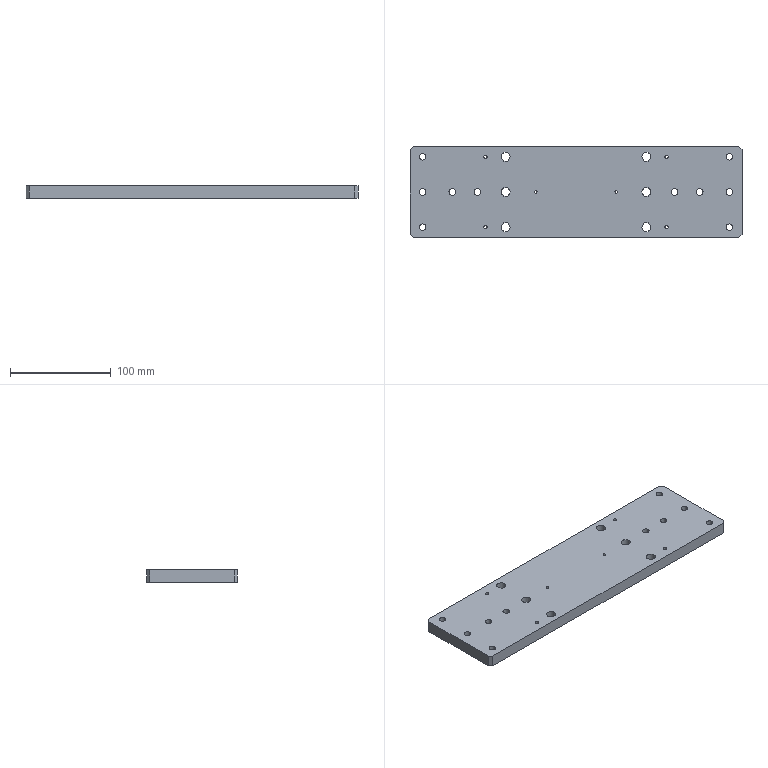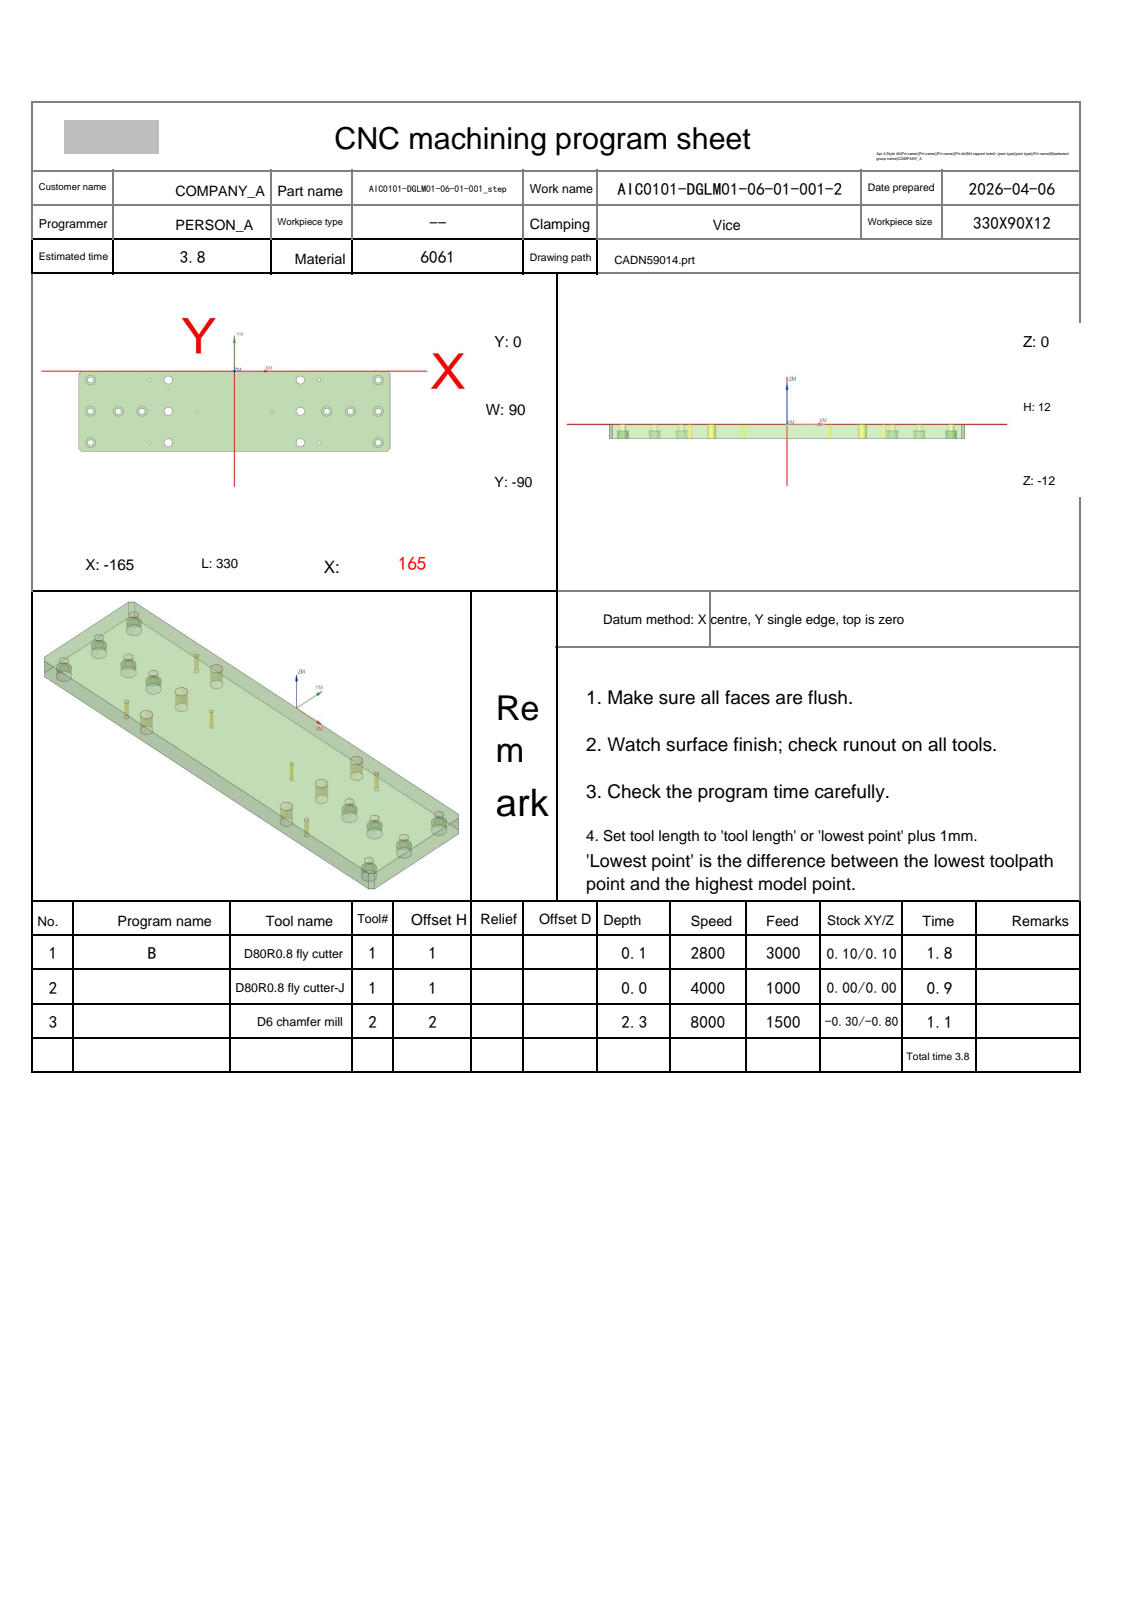NC program | NX | posted by the shop | part box 330 x 90 x 12 mm
Whole program:
%
O0001
(Machine time: 4.35 MIN)
(===Total Tool:2===)
(T1=D80R0.8 fly cutter D=80.  R=0.8  D-  H01 Z=0.    )
(T2=D6 chamfer mill   D=6.   R=0.   D-  H02 Z=-2.3  )
G80 G90 G17 G49 G40
G91 G28 Z0
M01
N1 T01 M06
(D80R0.8 fly cutter  D=80. R=0.8 H=01 ce=0.10 di=0.10)
G00 G90 G54 X-217.097 Y-23.903 M03 S2800
G43 H01 Z20.
M08
Z4.517
G01 Z2.517 F3000.
X-205.097
X197.897
G02 X205.097 Y-31.103 I0.0 J-7.2
G01 Y-50.737
G02 X197.097 Y-58.737 I-8. J0.0
G01 X-205.097
X-217.097
Z4.517
G00 Y-23.903
Z4.033
G01 Z2.033
X-205.097
X197.897
G02 X205.097 Y-31.103 I0.0 J-7.2
G01 Y-50.737
G02 X197.097 Y-58.737 I-8. J0.0
G01 X-205.097
X-217.097
Z4.033
G00 Y-23.903
Z3.55
G01 Z1.55
X-205.097
X197.897
G02 X205.097 Y-31.103 I0.0 J-7.2
G01 Y-50.737
G02 X197.097 Y-58.737 I-8. J0.0
G01 X-205.097
X-217.097
Z3.55
G00 Y-23.903
Z3.067
G01 Z1.067
X-205.097
X197.897
G02 X205.097 Y-31.103 I0.0 J-7.2
G01 Y-50.737
G02 X197.097 Y-58.737 I-8. J0.0
G01 X-205.097
X-217.097
Z3.067
G00 Y-23.903
Z2.583
G01 Z.583
X-205.097
X197.897
G02 X205.097 Y-31.103 I0.0 J-7.2
G01 Y-50.737
G02 X197.097 Y-58.737 I-8. J0.0
G01 X-205.097
X-217.097
Z2.583
G00 Y-23.903
Z2.1
G01 Z.1
X-205.097
X197.897
G02 X205.097 Y-31.103 I0.0 J-7.2
G01 Y-50.737
G02 X197.097 Y-58.737 I-8. J0.0
G01 X-205.097
X-217.097
Z2.1
G00 Z20.
G91 G28 Z0.0
M05
M09
G91 G28 Z0.0
M01
N2 T01 M06
(D80R0.8 fly cutter-J  D=80. R=0.8 H=01 ce=0.00 di=0.00)
G00 G90 G54 X-216.999 Y-24.001 M03 S4000
G43 H01 Z20.
M08
Z2.
G01 Z0.0 F1000.
X-204.999
X197.799
G02 X204.999 Y-31.201 I0.0 J-7.2
G01 Y-50.639
G02 X196.999 Y-58.639 I-8. J0.0
G01 X-204.999
X-216.999
Z2.
G00 Z20.
G91 G28 Z0.0
M05
M09
G91 G28 Z0.0
M01
N3 T02 M06
(D6 chamfer mill  D=6. R=0. H=02 ce=0.00 di=0.00)
G00 G90 G54 X-40. Y-45. M03 S8000
G43 H02 Z20.
M08
G98 G81 X-40. Y-45. Z-1.75 R3. F1000.
X40.
G80
G00 Z20.
G00 G90 X-90. Y-10. M03 S8000
Z20.
G98 G81 X-90. Y-10. Z-2.2 R3. F1000.
Y-80.
X90.
Y-10.
G80
G00 Z20.
G00 G90 X-151.993 Y-11.087 M03 S8000
Z20.
Z-.9
G01 Z-1.4 F1200.
X-151.8 Y-11.5
G03 X-150.3 Y-10. I0.0 J1.5
X-152.5 Y-7.8 I-2.2 J0.0
X-154.7 Y-10. I0.0 J-2.2
X-152.5 Y-12.2 I2.2 J0.0
X-150.3 Y-10. I0.0 J2.2
X-151.8 Y-8.5 I-1.5 J0.0
G01 X-151.993 Y-8.913
Z-.9
G00 Z20.
Y-46.087
Z-.9
G01 Z-1.4
X-151.8 Y-46.5
G03 X-150.3 Y-45. I0.0 J1.5
X-152.5 Y-42.8 I-2.2 J0.0
X-154.7 Y-45. I0.0 J-2.2
X-152.5 Y-47.2 I2.2 J0.0
X-150.3 Y-45. I0.0 J2.2
X-151.8 Y-43.5 I-1.5 J0.0
G01 X-151.993 Y-43.913
Z-.9
G00 Z20.
Y-81.087
Z-.9
G01 Z-1.4
X-151.8 Y-81.5
G03 X-150.3 Y-80. I0.0 J1.5
X-152.5 Y-77.8 I-2.2 J0.0
X-154.7 Y-80. I0.0 J-2.2
X-152.5 Y-82.2 I2.2 J0.0
X-150.3 Y-80. I0.0 J2.2
X-151.8 Y-78.5 I-1.5 J0.0
G01 X-151.993 Y-78.913
Z-.9
G00 Z20.
X-122.493 Y-46.087
Z-.9
G01 Z-1.4
X-122.3 Y-46.5
G03 X-120.8 Y-45. I0.0 J1.5
X-123. Y-42.8 I-2.2 J0.0
X-125.2 Y-45. I0.0 J-2.2
X-123. Y-47.2 I2.2 J0.0
X-120.8 Y-45. I0.0 J2.2
X-122.3 Y-43.5 I-1.5 J0.0
G01 X-122.493 Y-43.913
Z-.9
G00 Z20.
X-97.493 Y-46.087
Z-.9
G01 Z-1.4
X-97.3 Y-46.5
G03 X-95.8 Y-45. I0.0 J1.5
X-98. Y-42.8 I-2.2 J0.0
X-100.2 Y-45. I0.0 J-2.2
X-98. Y-47.2 I2.2 J0.0
X-95.8 Y-45. I0.0 J2.2
X-97.3 Y-43.5 I-1.5 J0.0
G01 X-97.493 Y-43.913
Z-.9
G00 Z20.
X98.507 Y-46.087
Z-.9
G01 Z-1.4
X98.7 Y-46.5
G03 X100.2 Y-45. I0.0 J1.5
X98. Y-42.8 I-2.2 J0.0
X95.8 Y-45. I0.0 J-2.2
X98. Y-47.2 I2.2 J0.0
X100.2 Y-45. I0.0 J2.2
X98.7 Y-43.5 I-1.5 J0.0
G01 X98.507 Y-43.913
Z-.9
G00 Z20.
X123.507 Y-46.087
Z-.9
G01 Z-1.4
X123.7 Y-46.5
G03 X125.2 Y-45. I0.0 J1.5
X123. Y-42.8 I-2.2 J0.0
X120.8 Y-45. I0.0 J-2.2
X123. Y-47.2 I2.2 J0.0
X125.2 Y-45. I0.0 J2.2
X123.7 Y-43.5 I-1.5 J0.0
G01 X123.507 Y-43.913
Z-.9
G00 Z20.
X153.007 Y-81.087
Z-.9
G01 Z-1.4
X153.2 Y-81.5
G03 X154.7 Y-80. I0.0 J1.5
X152.5 Y-77.8 I-2.2 J0.0
X150.3 Y-80. I0.0 J-2.2
X152.5 Y-82.2 I2.2 J0.0
X154.7 Y-80. I0.0 J2.2
X153.2 Y-78.5 I-1.5 J0.0
G01 X153.007 Y-78.913
Z-.9
G00 Z20.
Y-46.087
Z-.9
G01 Z-1.4
X153.2 Y-46.5
G03 X154.7 Y-45. I0.0 J1.5
X152.5 Y-42.8 I-2.2 J0.0
X150.3 Y-45. I0.0 J-2.2
X152.5 Y-47.2 I2.2 J0.0
X154.7 Y-45. I0.0 J2.2
X153.2 Y-43.5 I-1.5 J0.0
G01 X153.007 Y-43.913
Z-.9
G00 Z20.
Y-11.087
Z-.9
G01 Z-1.4
X153.2 Y-11.5
G03 X154.7 Y-10. I0.0 J1.5
X152.5 Y-7.8 I-2.2 J0.0
X150.3 Y-10. I0.0 J-2.2
X152.5 Y-12.2 I2.2 J0.0
X154.7 Y-10. I0.0 J2.2
X153.2 Y-8.5 I-1.5 J0.0
G01 X153.007 Y-8.913
Z-.9
G00 Z20.
G00 G90 X-70.001 Y-78.5 M03 S8000
Z20.
Z-1.8
G01 Z-2.3 F1200.
X-71.
G03 X-72.5 Y-80. I0.0 J-1.5
X-70. Y-82.5 I2.5 J0.0
X-67.5 Y-80. I0.0 J2.5
X-70. Y-77.5 I-2.5 J0.0
X-72.5 Y-80. I0.0 J-2.5
X-71. Y-81.5 I1.5 J0.0
G01 X-70.
Z-1.8
G00 Z20.
Y-43.5
Z-1.8
G01 Z-2.3
X-71.
G03 X-72.5 Y-45. I0.0 J-1.5
X-70. Y-47.5 I2.5 J0.0
X-67.5 Y-45. I0.0 J2.5
X-70. Y-42.5 I-2.5 J0.0
X-72.5 Y-45. I0.0 J-2.5
X-71. Y-46.5 I1.5 J0.0
G01 X-70.001
Z-1.8
G00 Z20.
X-70. Y-8.5
Z-1.8
G01 Z-2.3
X-71.
G03 X-72.5 Y-10. I0.0 J-1.5
X-70. Y-12.5 I2.5 J0.0
X-67.5 Y-10. I0.0 J2.5
X-70. Y-7.5 I-2.5 J0.0
X-72.5 Y-10. I0.0 J-2.5
X-71. Y-11.5 I1.5 J0.0
G01 X-70.001
Z-1.8
G00 Z20.
X70. Y-8.5
Z-1.8
G01 Z-2.3
X69.
G03 X67.5 Y-10. I0.0 J-1.5
X70. Y-12.5 I2.5 J0.0
X72.5 Y-10. I0.0 J2.5
X70. Y-7.5 I-2.5 J0.0
X67.5 Y-10. I0.0 J-2.5
X69. Y-11.5 I1.5 J0.0
G01 X69.999
Z-1.8
G00 Z20.
X70. Y-43.5
Z-1.8
G01 Z-2.3
X69.
G03 X67.5 Y-45. I0.0 J-1.5
X70. Y-47.5 I2.5 J0.0
X72.5 Y-45. I0.0 J2.5
X70. Y-42.5 I-2.5 J0.0
X67.5 Y-45. I0.0 J-2.5
X69. Y-46.5 I1.5 J0.0
G01 X69.999
Z-1.8
G00 Z20.
Y-78.5
Z-1.8
G01 Z-2.3
X69.
G03 X67.5 Y-80. I0.0 J-1.5
X70. Y-82.5 I2.5 J0.0
X72.5 Y-80. I0.0 J2.5
X70. Y-77.5 I-2.5 J0.0
X67.5 Y-80. I0.0 J-2.5
X69. Y-81.5 I1.5 J0.0
G01 X70.
Z-1.8
G00 Z20.
G00 G90 X-153.046 Y-90.7 M03 S7000
Z20.
Z2.5
G01 X-161.876 Z-.714 F1500.
X-161.953 Z-.742
X-162.16 Y-90.662 Z-.819
X-162.355 Y-90.581 Z-.895
X-162.528 Y-90.462 Z-.972
X-162.583 Y-90.407 Z-1.
X-165.407 Y-87.583
G02 X-165.7 Y-86.876 I.707 J.707
G01 Y-3.124
G02 X-165.407 Y-2.417 I1. J0.0
G01 X-162.583 Y.407
G02 X-161.876 Y.7 I.707 J-.707
G01 X161.876
G02 X162.583 Y.407 I0.0 J-1.
G01 X165.407 Y-2.417
G02 X165.7 Y-3.124 I-.707 J-.707
G01 Y-86.876
G02 X165.407 Y-87.583 I-1. J0.0
G01 X162.583 Y-90.407
G02 X161.876 Y-90.7 I-.707 J.707
G01 X-161.876
G02 X-162.583 Y-90.407 I0.0 J1.
G01 X-162.936 Y-90.054
Z1.5
G00 Z20.
M05
M09
G91 G28 Z0.0
G91 G28 Y0.0
M30
%